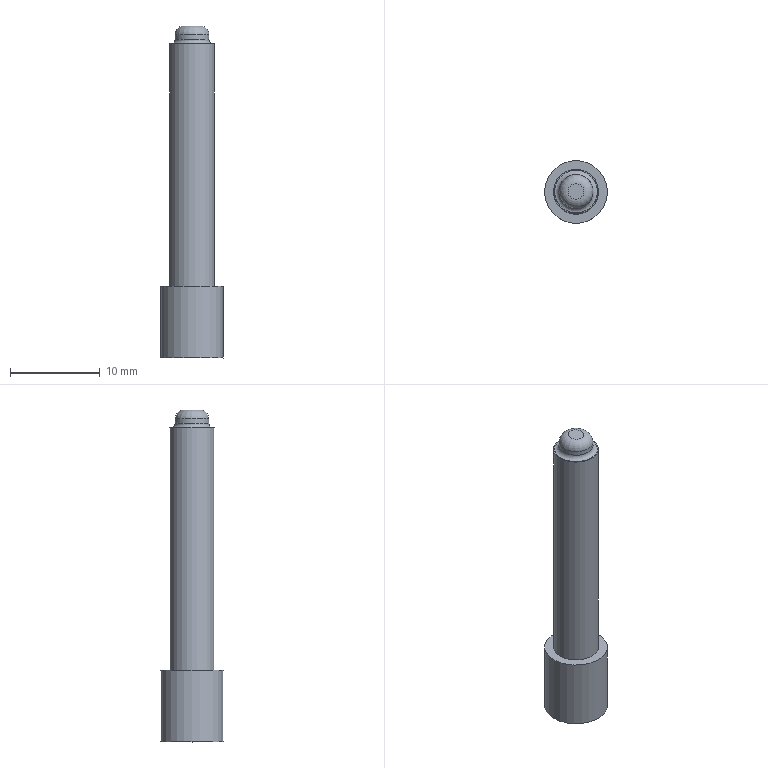Part | NX | features solid 2 | 1 solid | 9 faces | box 7 x 7 x 37 mm | volume 858.892 mm3 | plane 4 | cylinder 3 | torus 2 | commonest cylinder face diameters 3.78 x1 5 x1 7 x1
STEP:
#1=CARTESIAN_POINT('',(4211.736,-877.122,858.716));
#2=VERTEX_POINT('',#1);
#3=CARTESIAN_POINT('',(4209.236,-877.122,858.716));
#4=DIRECTION('',(0.,0.,1.));
#5=DIRECTION('',(1.,0.,0.));
#6=AXIS2_PLACEMENT_3D('',#3,#4,#5);
#7=CIRCLE('',#6,2.5);
#8=EDGE_CURVE('',#2,#2,#7,.T.);
#9=ORIENTED_EDGE('',*,*,#8,.F.);
#10=EDGE_LOOP('',(#9));
#11=FACE_BOUND('',#10,.T.);
#12=CARTESIAN_POINT('',(4206.736,-877.122,831.716));
#13=VERTEX_POINT('',#12);
#14=CARTESIAN_POINT('',(4209.236,-877.122,831.716));
#15=DIRECTION('',(0.,0.,-1.));
#16=DIRECTION('',(-1.,0.,0.));
#17=AXIS2_PLACEMENT_3D('',#14,#15,#16);
#18=CIRCLE('',#17,2.5);
#19=EDGE_CURVE('',#13,#13,#18,.F.);
#20=ORIENTED_EDGE('',*,*,#19,.T.);
#21=EDGE_LOOP('',(#20));
#22=FACE_BOUND('',#21,.T.);
#23=CARTESIAN_POINT('',(4209.236,-877.122,823.716));
#24=DIRECTION('',(0.,0.,1.));
#25=DIRECTION('',(1.,0.,0.));
#26=AXIS2_PLACEMENT_3D('',#23,#24,#25);
#27=CYLINDRICAL_SURFACE('',#26,2.5);
#28=ADVANCED_FACE('',(#11,#22),#27,.T.);
#29=CARTESIAN_POINT('',(4211.116,-876.924,859.716));
#30=VERTEX_POINT('',#29);
#31=CARTESIAN_POINT('',(4210.552,-875.492,859.716));
#32=CARTESIAN_POINT('',(4211.319,-876.903,859.716));
#33=CARTESIAN_POINT('',(4210.864,-878.44,859.716));
#34=CARTESIAN_POINT('',(4209.458,-879.205,859.716));
#35=CARTESIAN_POINT('',(4207.92,-878.752,859.716));
#36=CARTESIAN_POINT('',(4207.153,-877.343,859.716));
#37=CARTESIAN_POINT('',(4207.606,-875.807,859.716));
#38=CARTESIAN_POINT('',(4209.014,-875.04,859.716));
#39=CARTESIAN_POINT('',(4210.552,-875.492,859.716));
#40=CARTESIAN_POINT('',(4211.319,-876.903,859.716));
#41=CARTESIAN_POINT('',(4210.864,-878.44,859.716));
#42=B_SPLINE_CURVE_WITH_KNOTS('',3,(#31,#32,#33,#34,#35,#36,#37,#38,#39,#40,#41),.UNSPECIFIED.,.T.,.F.,(1,1,1,1,1,1,1,1,1,1,1,1,1,1,1),(-0.004431,-0.002954,-0.001477,0.,0.001477,0.002954,0.004431,0.005908,0.007385,0.008863,0.01034,0.01182,0.01329,0.01477,0.01625),.UNSPECIFIED.);
#43=EDGE_CURVE('',#30,#30,#42,.T.);
#44=ORIENTED_EDGE('',*,*,#43,.T.);
#45=EDGE_LOOP('',(#44));
#46=FACE_BOUND('',#45,.T.);
#47=CARTESIAN_POINT('',(4211.126,-877.122,859.216));
#48=VERTEX_POINT('',#47);
#49=CARTESIAN_POINT('',(4209.236,-877.122,859.216));
#50=DIRECTION('',(0.,0.,1.));
#51=DIRECTION('',(1.,0.,0.));
#52=AXIS2_PLACEMENT_3D('',#49,#50,#51);
#53=CIRCLE('',#52,1.89);
#54=EDGE_CURVE('',#48,#48,#53,.F.);
#55=ORIENTED_EDGE('',*,*,#54,.F.);
#56=EDGE_LOOP('',(#55));
#57=FACE_BOUND('',#56,.T.);
#58=CARTESIAN_POINT('',(4209.236,-877.122,860.716));
#59=DIRECTION('',(0.,0.,-1.));
#60=DIRECTION('',(-1.,0.,0.));
#61=AXIS2_PLACEMENT_3D('',#58,#59,#60);
#62=CYLINDRICAL_SURFACE('',#61,1.89);
#63=ADVANCED_FACE('',(#46,#57),#62,.T.);
#64=CARTESIAN_POINT('',(4208.346,-877.122,860.716));
#65=VERTEX_POINT('',#64);
#66=CARTESIAN_POINT('',(4209.236,-877.122,860.716));
#67=DIRECTION('',(0.,0.,-1.));
#68=DIRECTION('',(-1.,0.,0.));
#69=AXIS2_PLACEMENT_3D('',#66,#67,#68);
#70=CIRCLE('',#69,0.89);
#71=EDGE_CURVE('',#65,#65,#70,.F.);
#72=ORIENTED_EDGE('',*,*,#71,.T.);
#73=EDGE_LOOP('',(#72));
#74=FACE_BOUND('',#73,.T.);
#75=CARTESIAN_POINT('',(4209.236,-877.122,860.716));
#76=DIRECTION('',(0.,0.,-1.));
#77=DIRECTION('',(-1.,0.,0.));
#78=AXIS2_PLACEMENT_3D('',#75,#76,#77);
#79=PLANE('',#78);
#80=ADVANCED_FACE('',(#74),#79,.F.);
#81=CARTESIAN_POINT('',(4211.626,-877.122,858.716));
#82=VERTEX_POINT('',#81);
#83=CARTESIAN_POINT('',(4209.236,-877.122,858.716));
#84=DIRECTION('',(0.,0.,1.));
#85=DIRECTION('',(1.,0.,0.));
#86=AXIS2_PLACEMENT_3D('',#83,#84,#85);
#87=CIRCLE('',#86,2.39);
#88=EDGE_CURVE('',#82,#82,#87,.F.);
#89=ORIENTED_EDGE('',*,*,#88,.F.);
#90=EDGE_LOOP('',(#89));
#91=FACE_BOUND('',#90,.T.);
#92=ORIENTED_EDGE('',*,*,#54,.T.);
#93=EDGE_LOOP('',(#92));
#94=FACE_BOUND('',#93,.T.);
#95=CARTESIAN_POINT('',(4209.236,-877.122,859.216));
#96=DIRECTION('',(0.,0.,1.));
#97=DIRECTION('',(1.,0.,0.));
#98=AXIS2_PLACEMENT_3D('',#95,#96,#97);
#99=TOROIDAL_SURFACE('',#98,2.39,0.5);
#100=ADVANCED_FACE('',(#91,#94),#99,.F.);
#101=ORIENTED_EDGE('',*,*,#88,.T.);
#102=EDGE_LOOP('',(#101));
#103=FACE_BOUND('',#102,.T.);
#104=ORIENTED_EDGE('',*,*,#8,.T.);
#105=EDGE_LOOP('',(#104));
#106=FACE_BOUND('',#105,.T.);
#107=CARTESIAN_POINT('',(4217.236,-839.122,858.716));
#108=DIRECTION('',(0.,0.,1.));
#109=DIRECTION('',(1.,0.,0.));
#110=AXIS2_PLACEMENT_3D('',#107,#108,#109);
#111=PLANE('',#110);
#112=ADVANCED_FACE('',(#103,#106),#111,.T.);
#113=ORIENTED_EDGE('',*,*,#71,.F.);
#114=EDGE_LOOP('',(#113));
#115=FACE_BOUND('',#114,.T.);
#116=ORIENTED_EDGE('',*,*,#43,.F.);
#117=EDGE_LOOP('',(#116));
#118=FACE_BOUND('',#117,.T.);
#119=CARTESIAN_POINT('',(4209.236,-877.122,859.716));
#120=DIRECTION('',(0.,0.,-1.));
#121=DIRECTION('',(-1.,0.,0.));
#122=AXIS2_PLACEMENT_3D('',#119,#120,#121);
#123=DEGENERATE_TOROIDAL_SURFACE('',#122,0.89,1.,.T.);
#124=ADVANCED_FACE('',(#115,#118),#123,.T.);
#125=CARTESIAN_POINT('',(4205.736,-877.122,823.716));
#126=VERTEX_POINT('',#125);
#127=CARTESIAN_POINT('',(4209.236,-877.122,823.716));
#128=DIRECTION('',(0.,0.,-1.));
#129=DIRECTION('',(-1.,0.,0.));
#130=AXIS2_PLACEMENT_3D('',#127,#128,#129);
#131=CIRCLE('',#130,3.5);
#132=EDGE_CURVE('',#126,#126,#131,.F.);
#133=ORIENTED_EDGE('',*,*,#132,.F.);
#134=EDGE_LOOP('',(#133));
#135=FACE_BOUND('',#134,.T.);
#136=CARTESIAN_POINT('',(4209.236,-877.122,823.716));
#137=DIRECTION('',(0.,0.,-1.));
#138=DIRECTION('',(-1.,0.,0.));
#139=AXIS2_PLACEMENT_3D('',#136,#137,#138);
#140=PLANE('',#139);
#141=ADVANCED_FACE('',(#135),#140,.T.);
#142=CARTESIAN_POINT('',(4205.736,-877.122,831.716));
#143=VERTEX_POINT('',#142);
#144=CARTESIAN_POINT('',(4209.236,-877.122,831.716));
#145=DIRECTION('',(0.,0.,-1.));
#146=DIRECTION('',(-1.,0.,0.));
#147=AXIS2_PLACEMENT_3D('',#144,#145,#146);
#148=CIRCLE('',#147,3.5);
#149=EDGE_CURVE('',#143,#143,#148,.T.);
#150=ORIENTED_EDGE('',*,*,#149,.T.);
#151=EDGE_LOOP('',(#150));
#152=FACE_BOUND('',#151,.T.);
#153=ORIENTED_EDGE('',*,*,#132,.T.);
#154=EDGE_LOOP('',(#153));
#155=FACE_BOUND('',#154,.T.);
#156=CARTESIAN_POINT('',(4209.236,-877.122,823.716));
#157=DIRECTION('',(0.,0.,1.));
#158=DIRECTION('',(1.,0.,0.));
#159=AXIS2_PLACEMENT_3D('',#156,#157,#158);
#160=CYLINDRICAL_SURFACE('',#159,3.5);
#161=ADVANCED_FACE('',(#152,#155),#160,.T.);
#162=ORIENTED_EDGE('',*,*,#19,.F.);
#163=EDGE_LOOP('',(#162));
#164=FACE_BOUND('',#163,.T.);
#165=ORIENTED_EDGE('',*,*,#149,.F.);
#166=EDGE_LOOP('',(#165));
#167=FACE_BOUND('',#166,.T.);
#168=CARTESIAN_POINT('',(4217.236,-877.122,831.716));
#169=DIRECTION('',(0.,0.,-1.));
#170=DIRECTION('',(-1.,0.,0.));
#171=AXIS2_PLACEMENT_3D('',#168,#169,#170);
#172=PLANE('',#171);
#173=ADVANCED_FACE('',(#164,#167),#172,.F.);
#174=CLOSED_SHELL('',(#28,#63,#80,#100,#112,#124,#141,#161,#173));
#175=MANIFOLD_SOLID_BREP('',#174);
#176=(LENGTH_UNIT()NAMED_UNIT(*)SI_UNIT(.MILLI.,.METRE.));
#177=UNCERTAINTY_MEASURE_WITH_UNIT(LENGTH_MEASURE(0.0508),#176,'','');
#178=(NAMED_UNIT(*)PLANE_ANGLE_UNIT()SI_UNIT($,.RADIAN.));
#179=(NAMED_UNIT(*)SI_UNIT($,.STERADIAN.)SOLID_ANGLE_UNIT());
#180=(GEOMETRIC_REPRESENTATION_CONTEXT(3)GLOBAL_UNCERTAINTY_ASSIGNED_CONTEXT((#177))GLOBAL_UNIT_ASSIGNED_CONTEXT((#176,#178,#179))REPRESENTATION_CONTEXT('',''));
#181=ADVANCED_BREP_SHAPE_REPRESENTATION('',(#175),#180);